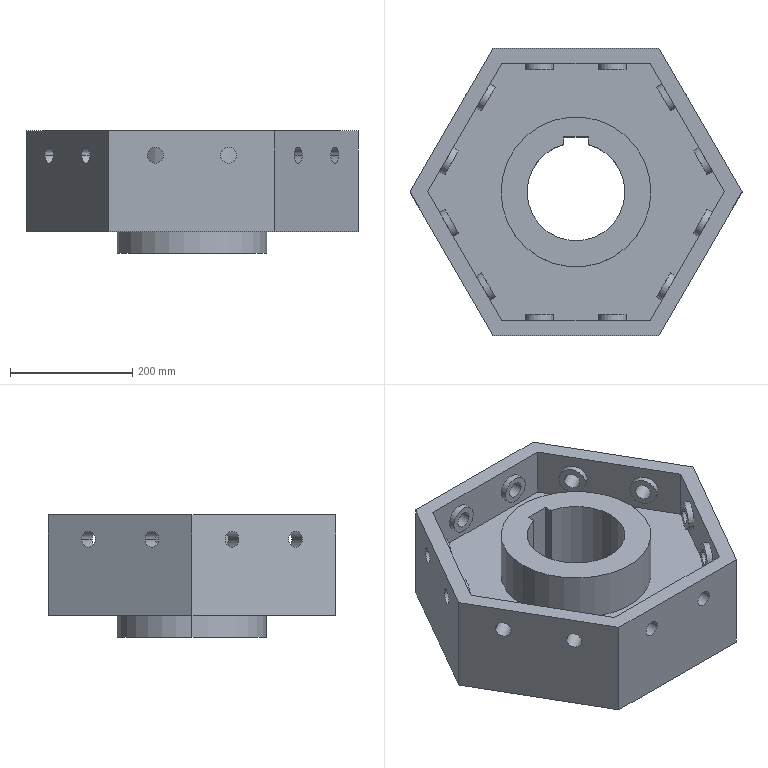Part | NX | features BREP 1 | 1 solid | 94 faces | box 542.709 x 470 x 200 mm | volume 14287973 mm3 | cylinder 55 | plane 39 | commonest cylinder face diameters 26 x24 45 x24 245 x4 160 x3